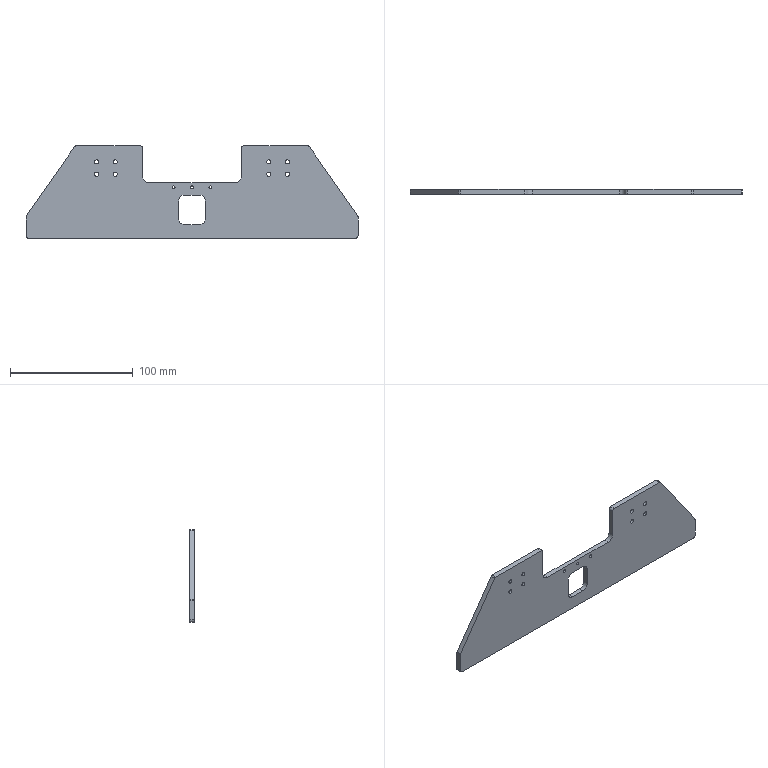Part | STEP file | side push plate | 1 solid | 52 faces | box 270 x 4 x 75 mm | volume 59912 mm3 | cylinder 36 | plane 16 | commonest cylinder face diameters 3.4 x16 4 x8 2.5 x6 10 x6